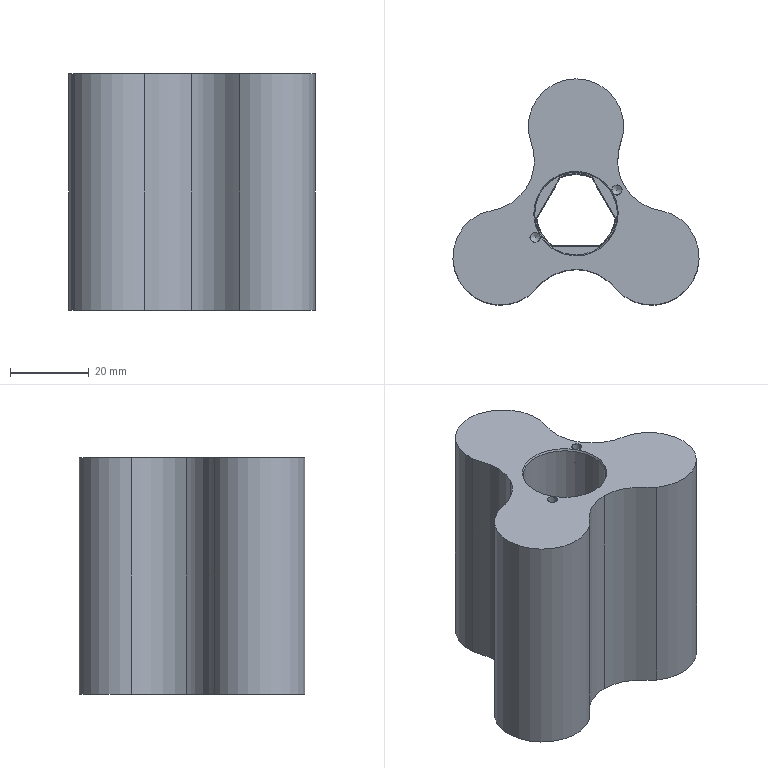CAM job | NX | 3-axis milling, drilling | part box 62.563 x 57.43 x 60 mm | stock box 72.563 x 72.563 x 60 mm
Tools:
number,name,description,diameter,corner_radius,flute_length,length,flutes
1,ZXZ,Milling Tool-5 Parameters,6.0,0.0,50.0,75.0,2
12,2.4ZT,Drilling Tool,2.5,0.0,35.0,50.0,2
13,2.5JD,Milling Tool-5 Parameters,2.5,0.0,50.0,75.0,2
12,D12,Milling Tool-5 Parameters,12.0,0.0,50.0,75.0,2
7,D6A45,Milling Tool-5 Parameters,6.0,0.0,50.0,75.0,2
5,D35R0.5,Milling Tool-5 Parameters,35.0,0.5,50.0,75.0,2
Operations:
program,operation,operation_type,tool,method,geometry_group,spindle_rpm,surface_speed,feed_per_tooth,feed_cut,feed_plunge,cut_length_mm,path_length_mm,cut_time_min,machine_time_min
1,DRILLING_COPY_1_COPY_1,Operation,ZXZ,METHOD,A,5000.0,94.0,0.025,250.0,0.0,8.0,103.187,0.032,0.0415
1,DRILLING_COPY_1_COPY_COPY_1,Operation,2.4ZT,METHOD,A,2000.0,15.0,0.03,120.0,0.0,15.502,118.191,0.1292,0.1395
1,DRILLING_COPY_1_COPY_COPY_COPY,Operation,2.5JD,METHOD,A,1000.0,9.0,0.025,50.0,0.0,14.0,115.187,0.28,0.2901
1,ZLEVEL_PROFILE_COPY_1_COPY,ZLevelMilling,D12,METHOD,A,3000.0,113.0,0.3,1800.0,1000.0,3524.546,3644.246,2.012,2.024
1,CUTTER_COMP_12_1_COPY,ZLevelMilling,D12,METHOD,A,5000.0,157.0,0.125,1250.0,100.0,1057.618,5475.333,0.8461,1.288
2,ZLEVEL_PROFILE,ZLevelMilling,D35R0.5,METHOD,A,2000.0,157.0,0.55,2200.0,1000.0,53824.485,53938.485,24.535,24.547
2,PLANAR_MILL_COPY_COPY_COPY,PlanarMilling,D6A45,METHOD,A,7500.0,141.0,0.0833,1250.0,100.0,223.347,280.348,0.1787,0.1844
2,CUTTER_COMP_12,ZLevelMilling,D12,METHOD,A,5000.0,157.0,0.125,1250.0,100.0,15396.009,15786.673,12.317,12.356